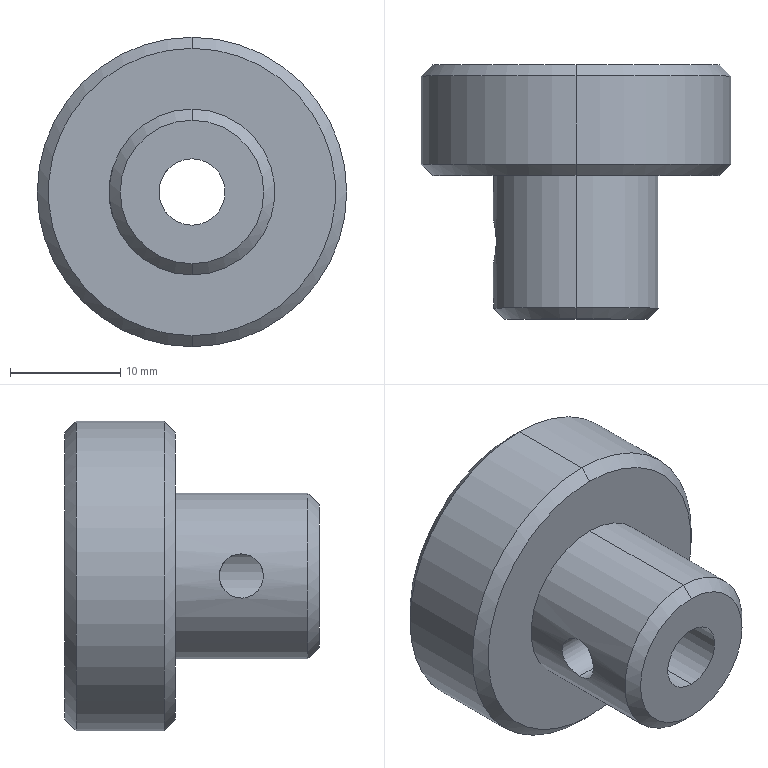Part | SolidWorks | features ICE 2, Chamfer 1, Extrusion 1 | 1 solid | 17 faces | box 28 x 23 x 28 mm | volume 7638 mm3 | cylinder 8 | cone 6 | plane 3 | commonest cylinder face diameters 4 x2 6 x2 15 x2 28 x2
STEP:
#1=CARTESIAN_POINT('',(-7.228,7.04,2.));
#2=VERTEX_POINT('',#1);
#3=CARTESIAN_POINT('',(-7.228,7.04,-2.));
#4=VERTEX_POINT('',#3);
#5=CARTESIAN_POINT('',(-7.228,7.04,2.));
#6=CARTESIAN_POINT('',(-7.228,6.778,2.));
#7=CARTESIAN_POINT('',(-7.244,6.514,1.947));
#8=CARTESIAN_POINT('',(-7.282,6.152,1.797));
#9=CARTESIAN_POINT('',(-7.297,6.035,1.734));
#10=CARTESIAN_POINT('',(-7.33,5.819,1.589));
#11=CARTESIAN_POINT('',(-7.348,5.718,1.507));
#12=CARTESIAN_POINT('',(-7.383,5.534,1.323));
#13=CARTESIAN_POINT('',(-7.401,5.45,1.22));
#14=CARTESIAN_POINT('',(-7.433,5.305,1.005));
#15=CARTESIAN_POINT('',(-7.448,5.244,0.8899));
#16=CARTESIAN_POINT('',(-7.473,5.142,0.6464));
#17=CARTESIAN_POINT('',(-7.483,5.104,0.5208));
#18=CARTESIAN_POINT('',(-7.496,5.053,0.2647));
#19=CARTESIAN_POINT('',(-7.5,5.04,0.1323));
#20=CARTESIAN_POINT('',(-7.5,5.04,-0.1314));
#21=CARTESIAN_POINT('',(-7.497,5.052,-0.2616));
#22=CARTESIAN_POINT('',(-7.483,5.104,-0.5188));
#23=CARTESIAN_POINT('',(-7.473,5.142,-0.6464));
#24=CARTESIAN_POINT('',(-7.436,5.293,-1.008));
#25=CARTESIAN_POINT('',(-7.401,5.441,-1.23));
#26=CARTESIAN_POINT('',(-7.348,5.717,-1.505));
#27=CARTESIAN_POINT('',(-7.33,5.818,-1.589));
#28=CARTESIAN_POINT('',(-7.297,6.036,-1.735));
#29=CARTESIAN_POINT('',(-7.282,6.15,-1.796));
#30=CARTESIAN_POINT('',(-7.256,6.391,-1.896));
#31=CARTESIAN_POINT('',(-7.246,6.519,-1.935));
#32=CARTESIAN_POINT('',(-7.232,6.776,-1.987));
#33=CARTESIAN_POINT('',(-7.228,6.907,-2.));
#34=CARTESIAN_POINT('',(-7.228,7.04,-2.));
#35=B_SPLINE_CURVE_WITH_KNOTS('',3,(#5,#6,#7,#8,#9,#10,#11,#12,#13,#14,#15,#16,#17,#18,#19,#20,#21,#22,#23,#24,#25,#26,#27,#28,#29,#30,#31,#32,#33,#34),.UNSPECIFIED.,.F.,.F.,(4,2,2,2,2,2,2,2,2,2,2,2,2,2,4),(0.006281,0.007066,0.007459,0.007851,0.008244,0.008636,0.009029,0.009421,0.009814,0.01021,0.01099,0.01138,0.01178,0.01217,0.01256),.UNSPECIFIED.);
#36=EDGE_CURVE('',#2,#4,#35,.T.);
#37=ORIENTED_EDGE('',*,*,#36,.F.);
#38=CARTESIAN_POINT('',(-2.236,7.04,2.));
#39=VERTEX_POINT('',#38);
#40=CARTESIAN_POINT('',(-15.,7.04,2.));
#41=DIRECTION('',(1.,0.,0.));
#42=VECTOR('',#41,1000.);
#43=LINE('',#40,#42);
#44=EDGE_CURVE('',#2,#39,#43,.T.);
#45=ORIENTED_EDGE('',*,*,#44,.T.);
#46=CARTESIAN_POINT('',(-2.236,7.04,-2.));
#47=VERTEX_POINT('',#46);
#48=CARTESIAN_POINT('',(-2.236,7.04,2.));
#49=CARTESIAN_POINT('',(-2.236,6.769,2.));
#50=CARTESIAN_POINT('',(-2.289,6.501,1.944));
#51=CARTESIAN_POINT('',(-2.446,6.022,1.741));
#52=CARTESIAN_POINT('',(-2.548,5.81,1.597));
#53=CARTESIAN_POINT('',(-2.692,5.539,1.329));
#54=CARTESIAN_POINT('',(-2.738,5.459,1.231));
#55=CARTESIAN_POINT('',(-2.823,5.315,1.02));
#56=CARTESIAN_POINT('',(-2.863,5.251,0.905));
#57=CARTESIAN_POINT('',(-2.928,5.148,0.6631));
#58=CARTESIAN_POINT('',(-2.955,5.108,0.5369));
#59=CARTESIAN_POINT('',(-2.991,5.054,0.2726));
#60=CARTESIAN_POINT('',(-3.,5.04,0.137));
#61=CARTESIAN_POINT('',(-3.,5.039,-0.1323));
#62=CARTESIAN_POINT('',(-2.991,5.053,-0.2692));
#63=CARTESIAN_POINT('',(-2.955,5.107,-0.5325));
#64=CARTESIAN_POINT('',(-2.929,5.147,-0.6592));
#65=CARTESIAN_POINT('',(-2.864,5.25,-0.9032));
#66=CARTESIAN_POINT('',(-2.825,5.313,-1.017));
#67=CARTESIAN_POINT('',(-2.739,5.457,-1.23));
#68=CARTESIAN_POINT('',(-2.691,5.54,-1.329));
#69=CARTESIAN_POINT('',(-2.596,5.719,-1.507));
#70=CARTESIAN_POINT('',(-2.547,5.816,-1.587));
#71=CARTESIAN_POINT('',(-2.453,6.028,-1.73));
#72=CARTESIAN_POINT('',(-2.407,6.141,-1.792));
#73=CARTESIAN_POINT('',(-2.329,6.379,-1.892));
#74=CARTESIAN_POINT('',(-2.295,6.506,-1.932));
#75=CARTESIAN_POINT('',(-2.249,6.769,-1.986));
#76=CARTESIAN_POINT('',(-2.236,6.903,-2.));
#77=CARTESIAN_POINT('',(-2.236,7.04,-2.));
#78=B_SPLINE_CURVE_WITH_KNOTS('',3,(#48,#49,#50,#51,#52,#53,#54,#55,#56,#57,#58,#59,#60,#61,#62,#63,#64,#65,#66,#67,#68,#69,#70,#71,#72,#73,#74,#75,#76,#77),.UNSPECIFIED.,.F.,.F.,(4,2,2,2,2,2,2,2,2,2,2,2,2,2,4),(0.00646,0.007265,0.00807,0.008472,0.008875,0.009277,0.00968,0.01008,0.01048,0.01089,0.01129,0.01169,0.0121,0.0125,0.0129),.UNSPECIFIED.);
#79=EDGE_CURVE('',#39,#47,#78,.T.);
#80=ORIENTED_EDGE('',*,*,#79,.T.);
#81=CARTESIAN_POINT('',(-15.,7.04,-2.));
#82=DIRECTION('',(1.,0.,0.));
#83=VECTOR('',#82,1000.);
#84=LINE('',#81,#83);
#85=EDGE_CURVE('',#4,#47,#84,.T.);
#86=ORIENTED_EDGE('',*,*,#85,.F.);
#87=EDGE_LOOP('',(#37,#45,#80,#86));
#88=FACE_OUTER_BOUND('',#87,.T.);
#89=CARTESIAN_POINT('',(-15.,7.04,0.));
#90=DIRECTION('',(1.,0.,0.));
#91=DIRECTION('',(0.,0.,-1.));
#92=AXIS2_PLACEMENT_3D('',#89,#90,#91);
#93=CYLINDRICAL_SURFACE('',#92,2.);
#94=ADVANCED_FACE('',(#88),#93,.F.);
#95=CARTESIAN_POINT('',(0.,0.,-6.5));
#96=VERTEX_POINT('',#95);
#97=CARTESIAN_POINT('',(0.,0.,6.5));
#98=VERTEX_POINT('',#97);
#99=CARTESIAN_POINT('',(0.,0.,0.));
#100=DIRECTION('',(0.,-1.,0.));
#101=DIRECTION('',(0.,0.,1.));
#102=AXIS2_PLACEMENT_3D('',#99,#100,#101);
#103=CIRCLE('',#102,6.5);
#104=EDGE_CURVE('',#96,#98,#103,.T.);
#105=ORIENTED_EDGE('',*,*,#104,.F.);
#106=CARTESIAN_POINT('',(0.,1.,-7.5));
#107=VERTEX_POINT('',#106);
#108=CARTESIAN_POINT('',(0.,1.,-7.5));
#109=DIRECTION('',(0.,0.7071,-0.7071));
#110=VECTOR('',#109,1000.);
#111=LINE('',#108,#110);
#112=EDGE_CURVE('',#96,#107,#111,.T.);
#113=ORIENTED_EDGE('',*,*,#112,.T.);
#114=CARTESIAN_POINT('',(0.,1.,7.5));
#115=VERTEX_POINT('',#114);
#116=CARTESIAN_POINT('',(0.,1.,0.));
#117=DIRECTION('',(0.,1.,0.));
#118=DIRECTION('',(0.,0.,1.));
#119=AXIS2_PLACEMENT_3D('',#116,#117,#118);
#120=CIRCLE('',#119,7.5);
#121=EDGE_CURVE('',#115,#107,#120,.T.);
#122=ORIENTED_EDGE('',*,*,#121,.F.);
#123=CARTESIAN_POINT('',(0.,1.,7.5));
#124=DIRECTION('',(0.,0.7071,0.7071));
#125=VECTOR('',#124,1000.);
#126=LINE('',#123,#125);
#127=EDGE_CURVE('',#98,#115,#126,.T.);
#128=ORIENTED_EDGE('',*,*,#127,.F.);
#129=EDGE_LOOP('',(#105,#113,#122,#128));
#130=FACE_OUTER_BOUND('',#129,.T.);
#131=CARTESIAN_POINT('',(0.,1.,0.));
#132=DIRECTION('',(0.,1.,0.));
#133=DIRECTION('',(0.,0.,1.));
#134=AXIS2_PLACEMENT_3D('',#131,#132,#133);
#135=CONICAL_SURFACE('',#134,7.5,0.7854);
#136=ADVANCED_FACE('',(#130),#135,.T.);
#137=CARTESIAN_POINT('',(0.,13.,-13.));
#138=VERTEX_POINT('',#137);
#139=CARTESIAN_POINT('',(0.,13.,13.));
#140=VERTEX_POINT('',#139);
#141=CARTESIAN_POINT('',(0.,13.,0.));
#142=DIRECTION('',(0.,-1.,0.));
#143=DIRECTION('',(0.,0.,1.));
#144=AXIS2_PLACEMENT_3D('',#141,#142,#143);
#145=CIRCLE('',#144,13.);
#146=EDGE_CURVE('',#138,#140,#145,.T.);
#147=ORIENTED_EDGE('',*,*,#146,.F.);
#148=CARTESIAN_POINT('',(0.,14.,-14.));
#149=VERTEX_POINT('',#148);
#150=CARTESIAN_POINT('',(0.,14.,-14.));
#151=DIRECTION('',(0.,0.7071,-0.7071));
#152=VECTOR('',#151,1000.);
#153=LINE('',#150,#152);
#154=EDGE_CURVE('',#138,#149,#153,.T.);
#155=ORIENTED_EDGE('',*,*,#154,.T.);
#156=CARTESIAN_POINT('',(0.,14.,14.));
#157=VERTEX_POINT('',#156);
#158=CARTESIAN_POINT('',(0.,14.,0.));
#159=DIRECTION('',(0.,1.,0.));
#160=DIRECTION('',(0.,0.,1.));
#161=AXIS2_PLACEMENT_3D('',#158,#159,#160);
#162=CIRCLE('',#161,14.);
#163=EDGE_CURVE('',#157,#149,#162,.T.);
#164=ORIENTED_EDGE('',*,*,#163,.F.);
#165=CARTESIAN_POINT('',(0.,14.,14.));
#166=DIRECTION('',(0.,0.7071,0.7071));
#167=VECTOR('',#166,1000.);
#168=LINE('',#165,#167);
#169=EDGE_CURVE('',#140,#157,#168,.T.);
#170=ORIENTED_EDGE('',*,*,#169,.F.);
#171=EDGE_LOOP('',(#147,#155,#164,#170));
#172=FACE_OUTER_BOUND('',#171,.T.);
#173=CARTESIAN_POINT('',(0.,14.,0.));
#174=DIRECTION('',(0.,1.,0.));
#175=DIRECTION('',(0.,0.,1.));
#176=AXIS2_PLACEMENT_3D('',#173,#174,#175);
#177=CONICAL_SURFACE('',#176,14.,0.7854);
#178=ADVANCED_FACE('',(#172),#177,.T.);
#179=CARTESIAN_POINT('',(0.,23.,13.));
#180=VERTEX_POINT('',#179);
#181=CARTESIAN_POINT('',(0.,23.,-13.));
#182=VERTEX_POINT('',#181);
#183=CARTESIAN_POINT('',(0.,23.,0.));
#184=DIRECTION('',(0.,1.,0.));
#185=DIRECTION('',(0.,0.,1.));
#186=AXIS2_PLACEMENT_3D('',#183,#184,#185);
#187=CIRCLE('',#186,13.);
#188=EDGE_CURVE('',#180,#182,#187,.T.);
#189=ORIENTED_EDGE('',*,*,#188,.F.);
#190=CARTESIAN_POINT('',(0.,22.,14.));
#191=VERTEX_POINT('',#190);
#192=CARTESIAN_POINT('',(0.,23.,13.));
#193=DIRECTION('',(0.,-0.7071,0.7071));
#194=VECTOR('',#193,1000.);
#195=LINE('',#192,#194);
#196=EDGE_CURVE('',#180,#191,#195,.T.);
#197=ORIENTED_EDGE('',*,*,#196,.T.);
#198=CARTESIAN_POINT('',(0.,22.,-14.));
#199=VERTEX_POINT('',#198);
#200=CARTESIAN_POINT('',(0.,22.,0.));
#201=DIRECTION('',(0.,-1.,0.));
#202=DIRECTION('',(0.,0.,1.));
#203=AXIS2_PLACEMENT_3D('',#200,#201,#202);
#204=CIRCLE('',#203,14.);
#205=EDGE_CURVE('',#199,#191,#204,.T.);
#206=ORIENTED_EDGE('',*,*,#205,.F.);
#207=CARTESIAN_POINT('',(0.,23.,-13.));
#208=DIRECTION('',(0.,-0.7071,-0.7071));
#209=VECTOR('',#208,1000.);
#210=LINE('',#207,#209);
#211=EDGE_CURVE('',#182,#199,#210,.T.);
#212=ORIENTED_EDGE('',*,*,#211,.F.);
#213=EDGE_LOOP('',(#189,#197,#206,#212));
#214=FACE_OUTER_BOUND('',#213,.T.);
#215=CARTESIAN_POINT('',(0.,23.,0.));
#216=DIRECTION('',(0.,-1.,0.));
#217=DIRECTION('',(0.,0.,-1.));
#218=AXIS2_PLACEMENT_3D('',#215,#216,#217);
#219=CONICAL_SURFACE('',#218,13.,0.7854);
#220=ADVANCED_FACE('',(#214),#219,.T.);
#221=ORIENTED_EDGE('',*,*,#163,.T.);
#222=CARTESIAN_POINT('',(0.,13.,-14.));
#223=DIRECTION('',(0.,1.,0.));
#224=VECTOR('',#223,1000.);
#225=LINE('',#222,#224);
#226=EDGE_CURVE('',#149,#199,#225,.T.);
#227=ORIENTED_EDGE('',*,*,#226,.T.);
#228=ORIENTED_EDGE('',*,*,#205,.T.);
#229=CARTESIAN_POINT('',(0.,13.,14.));
#230=DIRECTION('',(0.,1.,0.));
#231=VECTOR('',#230,1000.);
#232=LINE('',#229,#231);
#233=EDGE_CURVE('',#157,#191,#232,.T.);
#234=ORIENTED_EDGE('',*,*,#233,.F.);
#235=EDGE_LOOP('',(#221,#227,#228,#234));
#236=FACE_OUTER_BOUND('',#235,.T.);
#237=CARTESIAN_POINT('',(0.,13.,0.));
#238=DIRECTION('',(0.,1.,0.));
#239=DIRECTION('',(0.,0.,1.));
#240=AXIS2_PLACEMENT_3D('',#237,#238,#239);
#241=CYLINDRICAL_SURFACE('',#240,14.);
#242=ADVANCED_FACE('',(#236),#241,.T.);
#243=CARTESIAN_POINT('',(-2.236,7.04,-2.));
#244=CARTESIAN_POINT('',(-2.236,7.177,-2.));
#245=CARTESIAN_POINT('',(-2.249,7.31,-1.986));
#246=CARTESIAN_POINT('',(-2.295,7.571,-1.933));
#247=CARTESIAN_POINT('',(-2.328,7.698,-1.893));
#248=CARTESIAN_POINT('',(-2.446,8.056,-1.742));
#249=CARTESIAN_POINT('',(-2.547,8.269,-1.597));
#250=CARTESIAN_POINT('',(-2.691,8.539,-1.33));
#251=CARTESIAN_POINT('',(-2.738,8.621,-1.231));
#252=CARTESIAN_POINT('',(-2.824,8.765,-1.019));
#253=CARTESIAN_POINT('',(-2.863,8.827,-0.9064));
#254=CARTESIAN_POINT('',(-2.928,8.93,-0.6656));
#255=CARTESIAN_POINT('',(-2.955,8.971,-0.5362));
#256=CARTESIAN_POINT('',(-2.99,9.025,-0.275));
#257=CARTESIAN_POINT('',(-3.,9.039,-0.1417));
#258=CARTESIAN_POINT('',(-3.,9.04,0.1311));
#259=CARTESIAN_POINT('',(-2.991,9.026,0.2667));
#260=CARTESIAN_POINT('',(-2.956,8.973,0.5294));
#261=CARTESIAN_POINT('',(-2.929,8.933,0.6589));
#262=CARTESIAN_POINT('',(-2.832,8.779,1.022));
#263=CARTESIAN_POINT('',(-2.74,8.63,1.238));
#264=CARTESIAN_POINT('',(-2.596,8.361,1.507));
#265=CARTESIAN_POINT('',(-2.547,8.262,1.588));
#266=CARTESIAN_POINT('',(-2.453,8.052,1.73));
#267=CARTESIAN_POINT('',(-2.408,7.94,1.791));
#268=CARTESIAN_POINT('',(-2.329,7.701,1.892));
#269=CARTESIAN_POINT('',(-2.295,7.574,1.932));
#270=CARTESIAN_POINT('',(-2.249,7.312,1.986));
#271=CARTESIAN_POINT('',(-2.236,7.175,2.));
#272=CARTESIAN_POINT('',(-2.236,7.04,2.));
#273=B_SPLINE_CURVE_WITH_KNOTS('',3,(#243,#244,#245,#246,#247,#248,#249,#250,#251,#252,#253,#254,#255,#256,#257,#258,#259,#260,#261,#262,#263,#264,#265,#266,#267,#268,#269,#270,#271,#272),.UNSPECIFIED.,.F.,.F.,(4,2,2,2,2,2,2,2,2,2,2,2,2,2,4),(0.,0.0004037,0.0008075,0.001615,0.002019,0.002422,0.002826,0.00323,0.003634,0.004037,0.004845,0.005248,0.005652,0.006056,0.00646),.UNSPECIFIED.);
#274=EDGE_CURVE('',#47,#39,#273,.T.);
#275=ORIENTED_EDGE('',*,*,#274,.F.);
#276=ORIENTED_EDGE('',*,*,#79,.F.);
#277=EDGE_LOOP('',(#275,#276));
#278=FACE_BOUND('',#277,.T.);
#279=CARTESIAN_POINT('',(0.,23.,-3.));
#280=VERTEX_POINT('',#279);
#281=CARTESIAN_POINT('',(0.,23.,3.));
#282=VERTEX_POINT('',#281);
#283=CARTESIAN_POINT('',(0.,23.,0.));
#284=DIRECTION('',(0.,1.,0.));
#285=DIRECTION('',(0.,0.,1.));
#286=AXIS2_PLACEMENT_3D('',#283,#284,#285);
#287=CIRCLE('',#286,3.);
#288=EDGE_CURVE('',#280,#282,#287,.T.);
#289=ORIENTED_EDGE('',*,*,#288,.T.);
#290=CARTESIAN_POINT('',(0.,0.,3.));
#291=VERTEX_POINT('',#290);
#292=CARTESIAN_POINT('',(0.,23.,3.));
#293=DIRECTION('',(0.,-1.,0.));
#294=VECTOR('',#293,1000.);
#295=LINE('',#292,#294);
#296=EDGE_CURVE('',#282,#291,#295,.T.);
#297=ORIENTED_EDGE('',*,*,#296,.T.);
#298=CARTESIAN_POINT('',(0.,0.,-3.));
#299=VERTEX_POINT('',#298);
#300=CARTESIAN_POINT('',(0.,0.,0.));
#301=DIRECTION('',(0.,1.,0.));
#302=DIRECTION('',(0.,0.,1.));
#303=AXIS2_PLACEMENT_3D('',#300,#301,#302);
#304=CIRCLE('',#303,3.);
#305=EDGE_CURVE('',#299,#291,#304,.T.);
#306=ORIENTED_EDGE('',*,*,#305,.F.);
#307=CARTESIAN_POINT('',(0.,23.,-3.));
#308=DIRECTION('',(0.,-1.,0.));
#309=VECTOR('',#308,1000.);
#310=LINE('',#307,#309);
#311=EDGE_CURVE('',#280,#299,#310,.T.);
#312=ORIENTED_EDGE('',*,*,#311,.F.);
#313=EDGE_LOOP('',(#289,#297,#306,#312));
#314=FACE_OUTER_BOUND('',#313,.T.);
#315=CARTESIAN_POINT('',(0.,23.,0.));
#316=DIRECTION('',(0.,-1.,0.));
#317=DIRECTION('',(0.,0.,-1.));
#318=AXIS2_PLACEMENT_3D('',#315,#316,#317);
#319=CYLINDRICAL_SURFACE('',#318,3.);
#320=ADVANCED_FACE('',(#278,#314),#319,.F.);
#321=CARTESIAN_POINT('',(0.,13.,7.5));
#322=VERTEX_POINT('',#321);
#323=CARTESIAN_POINT('',(0.,13.,-7.5));
#324=VERTEX_POINT('',#323);
#325=CARTESIAN_POINT('',(0.,13.,0.));
#326=DIRECTION('',(0.,1.,0.));
#327=DIRECTION('',(0.,0.,1.));
#328=AXIS2_PLACEMENT_3D('',#325,#326,#327);
#329=CIRCLE('',#328,7.5);
#330=EDGE_CURVE('',#322,#324,#329,.T.);
#331=ORIENTED_EDGE('',*,*,#330,.F.);
#332=CARTESIAN_POINT('',(0.,23.,7.5));
#333=DIRECTION('',(0.,-1.,0.));
#334=VECTOR('',#333,1000.);
#335=LINE('',#332,#334);
#336=EDGE_CURVE('',#322,#115,#335,.T.);
#337=ORIENTED_EDGE('',*,*,#336,.T.);
#338=ORIENTED_EDGE('',*,*,#121,.T.);
#339=CARTESIAN_POINT('',(0.,23.,-7.5));
#340=DIRECTION('',(0.,-1.,0.));
#341=VECTOR('',#340,1000.);
#342=LINE('',#339,#341);
#343=EDGE_CURVE('',#324,#107,#342,.T.);
#344=ORIENTED_EDGE('',*,*,#343,.F.);
#345=EDGE_LOOP('',(#331,#337,#338,#344));
#346=FACE_OUTER_BOUND('',#345,.T.);
#347=CARTESIAN_POINT('',(0.,23.,0.));
#348=DIRECTION('',(0.,-1.,0.));
#349=DIRECTION('',(0.,0.,-1.));
#350=AXIS2_PLACEMENT_3D('',#347,#348,#349);
#351=CYLINDRICAL_SURFACE('',#350,7.5);
#352=ADVANCED_FACE('',(#346),#351,.T.);
#353=ORIENTED_EDGE('',*,*,#336,.F.);
#354=CARTESIAN_POINT('',(0.,13.,0.));
#355=DIRECTION('',(0.,1.,0.));
#356=DIRECTION('',(0.,0.,1.));
#357=AXIS2_PLACEMENT_3D('',#354,#355,#356);
#358=CIRCLE('',#357,7.5);
#359=EDGE_CURVE('',#324,#322,#358,.T.);
#360=ORIENTED_EDGE('',*,*,#359,.F.);
#361=ORIENTED_EDGE('',*,*,#343,.T.);
#362=CARTESIAN_POINT('',(0.,1.,0.));
#363=DIRECTION('',(0.,1.,0.));
#364=DIRECTION('',(0.,0.,1.));
#365=AXIS2_PLACEMENT_3D('',#362,#363,#364);
#366=CIRCLE('',#365,7.5);
#367=EDGE_CURVE('',#107,#115,#366,.T.);
#368=ORIENTED_EDGE('',*,*,#367,.T.);
#369=EDGE_LOOP('',(#353,#360,#361,#368));
#370=FACE_OUTER_BOUND('',#369,.T.);
#371=CARTESIAN_POINT('',(-7.228,7.04,-2.));
#372=CARTESIAN_POINT('',(-7.228,7.172,-2.));
#373=CARTESIAN_POINT('',(-7.232,7.303,-1.987));
#374=CARTESIAN_POINT('',(-7.246,7.559,-1.936));
#375=CARTESIAN_POINT('',(-7.256,7.687,-1.897));
#376=CARTESIAN_POINT('',(-7.282,7.929,-1.796));
#377=CARTESIAN_POINT('',(-7.297,8.043,-1.735));
#378=CARTESIAN_POINT('',(-7.33,8.26,-1.59));
#379=CARTESIAN_POINT('',(-7.348,8.362,-1.506));
#380=CARTESIAN_POINT('',(-7.401,8.638,-1.23));
#381=CARTESIAN_POINT('',(-7.436,8.787,-1.008));
#382=CARTESIAN_POINT('',(-7.473,8.936,-0.6474));
#383=CARTESIAN_POINT('',(-7.483,8.975,-0.5206));
#384=CARTESIAN_POINT('',(-7.497,9.027,-0.2622));
#385=CARTESIAN_POINT('',(-7.5,9.04,-0.132));
#386=CARTESIAN_POINT('',(-7.5,9.04,0.1303));
#387=CARTESIAN_POINT('',(-7.496,9.027,0.2635));
#388=CARTESIAN_POINT('',(-7.483,8.975,0.5205));
#389=CARTESIAN_POINT('',(-7.473,8.937,0.6455));
#390=CARTESIAN_POINT('',(-7.436,8.786,1.01));
#391=CARTESIAN_POINT('',(-7.401,8.638,1.23));
#392=CARTESIAN_POINT('',(-7.348,8.361,1.507));
#393=CARTESIAN_POINT('',(-7.33,8.26,1.59));
#394=CARTESIAN_POINT('',(-7.297,8.044,1.734));
#395=CARTESIAN_POINT('',(-7.282,7.927,1.797));
#396=CARTESIAN_POINT('',(-7.256,7.686,1.897));
#397=CARTESIAN_POINT('',(-7.246,7.561,1.935));
#398=CARTESIAN_POINT('',(-7.232,7.303,1.987));
#399=CARTESIAN_POINT('',(-7.228,7.171,2.));
#400=CARTESIAN_POINT('',(-7.228,7.04,2.));
#401=B_SPLINE_CURVE_WITH_KNOTS('',3,(#371,#372,#373,#374,#375,#376,#377,#378,#379,#380,#381,#382,#383,#384,#385,#386,#387,#388,#389,#390,#391,#392,#393,#394,#395,#396,#397,#398,#399,#400),.UNSPECIFIED.,.F.,.F.,(4,2,2,2,2,2,2,2,2,2,2,2,2,2,4),(0.,0.0003926,0.0007852,0.001178,0.00157,0.002356,0.002748,0.003141,0.003533,0.003926,0.004711,0.005104,0.005496,0.005889,0.006281),.UNSPECIFIED.);
#402=EDGE_CURVE('',#4,#2,#401,.T.);
#403=ORIENTED_EDGE('',*,*,#402,.T.);
#404=ORIENTED_EDGE('',*,*,#36,.T.);
#405=EDGE_LOOP('',(#403,#404));
#406=FACE_BOUND('',#405,.T.);
#407=CARTESIAN_POINT('',(0.,23.,0.));
#408=DIRECTION('',(0.,-1.,0.));
#409=DIRECTION('',(0.,0.,-1.));
#410=AXIS2_PLACEMENT_3D('',#407,#408,#409);
#411=CYLINDRICAL_SURFACE('',#410,7.5);
#412=ADVANCED_FACE('',(#370,#406),#411,.T.);
#413=CARTESIAN_POINT('',(0.,23.,0.));
#414=DIRECTION('',(0.,1.,0.));
#415=DIRECTION('',(0.,0.,1.));
#416=AXIS2_PLACEMENT_3D('',#413,#414,#415);
#417=CIRCLE('',#416,13.);
#418=EDGE_CURVE('',#182,#180,#417,.T.);
#419=ORIENTED_EDGE('',*,*,#418,.T.);
#420=ORIENTED_EDGE('',*,*,#188,.T.);
#421=EDGE_LOOP('',(#419,#420));
#422=FACE_OUTER_BOUND('',#421,.T.);
#423=ORIENTED_EDGE('',*,*,#288,.F.);
#424=CARTESIAN_POINT('',(0.,23.,0.));
#425=DIRECTION('',(0.,1.,0.));
#426=DIRECTION('',(0.,0.,1.));
#427=AXIS2_PLACEMENT_3D('',#424,#425,#426);
#428=CIRCLE('',#427,3.);
#429=EDGE_CURVE('',#282,#280,#428,.T.);
#430=ORIENTED_EDGE('',*,*,#429,.F.);
#431=EDGE_LOOP('',(#423,#430));
#432=FACE_BOUND('',#431,.T.);
#433=CARTESIAN_POINT('',(0.,23.,0.));
#434=DIRECTION('',(0.,1.,0.));
#435=DIRECTION('',(0.,0.,1.));
#436=AXIS2_PLACEMENT_3D('',#433,#434,#435);
#437=PLANE('',#436);
#438=ADVANCED_FACE('',(#422,#432),#437,.T.);
#439=CARTESIAN_POINT('',(0.,0.,0.));
#440=DIRECTION('',(0.,-1.,0.));
#441=DIRECTION('',(0.,0.,1.));
#442=AXIS2_PLACEMENT_3D('',#439,#440,#441);
#443=CIRCLE('',#442,6.5);
#444=EDGE_CURVE('',#98,#96,#443,.T.);
#445=ORIENTED_EDGE('',*,*,#444,.T.);
#446=ORIENTED_EDGE('',*,*,#104,.T.);
#447=EDGE_LOOP('',(#445,#446));
#448=FACE_OUTER_BOUND('',#447,.T.);
#449=ORIENTED_EDGE('',*,*,#305,.T.);
#450=CARTESIAN_POINT('',(0.,0.,0.));
#451=DIRECTION('',(0.,1.,0.));
#452=DIRECTION('',(0.,0.,1.));
#453=AXIS2_PLACEMENT_3D('',#450,#451,#452);
#454=CIRCLE('',#453,3.);
#455=EDGE_CURVE('',#291,#299,#454,.T.);
#456=ORIENTED_EDGE('',*,*,#455,.T.);
#457=EDGE_LOOP('',(#449,#456));
#458=FACE_BOUND('',#457,.T.);
#459=CARTESIAN_POINT('',(0.,0.,0.));
#460=DIRECTION('',(0.,1.,0.));
#461=DIRECTION('',(0.,0.,1.));
#462=AXIS2_PLACEMENT_3D('',#459,#460,#461);
#463=PLANE('',#462);
#464=ADVANCED_FACE('',(#448,#458),#463,.F.);
#465=ORIENTED_EDGE('',*,*,#296,.F.);
#466=ORIENTED_EDGE('',*,*,#429,.T.);
#467=ORIENTED_EDGE('',*,*,#311,.T.);
#468=ORIENTED_EDGE('',*,*,#455,.F.);
#469=EDGE_LOOP('',(#465,#466,#467,#468));
#470=FACE_OUTER_BOUND('',#469,.T.);
#471=CARTESIAN_POINT('',(0.,23.,0.));
#472=DIRECTION('',(0.,-1.,0.));
#473=DIRECTION('',(0.,0.,-1.));
#474=AXIS2_PLACEMENT_3D('',#471,#472,#473);
#475=CYLINDRICAL_SURFACE('',#474,3.);
#476=ADVANCED_FACE('',(#470),#475,.F.);
#477=CARTESIAN_POINT('',(0.,13.,0.));
#478=DIRECTION('',(0.,-1.,0.));
#479=DIRECTION('',(0.,0.,1.));
#480=AXIS2_PLACEMENT_3D('',#477,#478,#479);
#481=CIRCLE('',#480,13.);
#482=EDGE_CURVE('',#140,#138,#481,.T.);
#483=ORIENTED_EDGE('',*,*,#482,.T.);
#484=ORIENTED_EDGE('',*,*,#146,.T.);
#485=EDGE_LOOP('',(#483,#484));
#486=FACE_OUTER_BOUND('',#485,.T.);
#487=ORIENTED_EDGE('',*,*,#359,.T.);
#488=ORIENTED_EDGE('',*,*,#330,.T.);
#489=EDGE_LOOP('',(#487,#488));
#490=FACE_BOUND('',#489,.T.);
#491=CARTESIAN_POINT('',(0.,13.,0.));
#492=DIRECTION('',(0.,1.,0.));
#493=DIRECTION('',(0.,0.,1.));
#494=AXIS2_PLACEMENT_3D('',#491,#492,#493);
#495=PLANE('',#494);
#496=ADVANCED_FACE('',(#486,#490),#495,.F.);
#497=ORIENTED_EDGE('',*,*,#226,.F.);
#498=CARTESIAN_POINT('',(0.,14.,0.));
#499=DIRECTION('',(0.,1.,0.));
#500=DIRECTION('',(0.,0.,1.));
#501=AXIS2_PLACEMENT_3D('',#498,#499,#500);
#502=CIRCLE('',#501,14.);
#503=EDGE_CURVE('',#149,#157,#502,.T.);
#504=ORIENTED_EDGE('',*,*,#503,.T.);
#505=ORIENTED_EDGE('',*,*,#233,.T.);
#506=CARTESIAN_POINT('',(0.,22.,0.));
#507=DIRECTION('',(0.,-1.,0.));
#508=DIRECTION('',(0.,0.,1.));
#509=AXIS2_PLACEMENT_3D('',#506,#507,#508);
#510=CIRCLE('',#509,14.);
#511=EDGE_CURVE('',#191,#199,#510,.T.);
#512=ORIENTED_EDGE('',*,*,#511,.T.);
#513=EDGE_LOOP('',(#497,#504,#505,#512));
#514=FACE_OUTER_BOUND('',#513,.T.);
#515=CARTESIAN_POINT('',(0.,13.,0.));
#516=DIRECTION('',(0.,1.,0.));
#517=DIRECTION('',(0.,0.,1.));
#518=AXIS2_PLACEMENT_3D('',#515,#516,#517);
#519=CYLINDRICAL_SURFACE('',#518,14.);
#520=ADVANCED_FACE('',(#514),#519,.T.);
#521=ORIENTED_EDGE('',*,*,#196,.F.);
#522=ORIENTED_EDGE('',*,*,#418,.F.);
#523=ORIENTED_EDGE('',*,*,#211,.T.);
#524=ORIENTED_EDGE('',*,*,#511,.F.);
#525=EDGE_LOOP('',(#521,#522,#523,#524));
#526=FACE_OUTER_BOUND('',#525,.T.);
#527=CARTESIAN_POINT('',(0.,23.,0.));
#528=DIRECTION('',(0.,-1.,0.));
#529=DIRECTION('',(0.,0.,-1.));
#530=AXIS2_PLACEMENT_3D('',#527,#528,#529);
#531=CONICAL_SURFACE('',#530,13.,0.7854);
#532=ADVANCED_FACE('',(#526),#531,.T.);
#533=ORIENTED_EDGE('',*,*,#154,.F.);
#534=ORIENTED_EDGE('',*,*,#482,.F.);
#535=ORIENTED_EDGE('',*,*,#169,.T.);
#536=ORIENTED_EDGE('',*,*,#503,.F.);
#537=EDGE_LOOP('',(#533,#534,#535,#536));
#538=FACE_OUTER_BOUND('',#537,.T.);
#539=CARTESIAN_POINT('',(0.,14.,0.));
#540=DIRECTION('',(0.,1.,0.));
#541=DIRECTION('',(0.,0.,1.));
#542=AXIS2_PLACEMENT_3D('',#539,#540,#541);
#543=CONICAL_SURFACE('',#542,14.,0.7854);
#544=ADVANCED_FACE('',(#538),#543,.T.);
#545=ORIENTED_EDGE('',*,*,#112,.F.);
#546=ORIENTED_EDGE('',*,*,#444,.F.);
#547=ORIENTED_EDGE('',*,*,#127,.T.);
#548=ORIENTED_EDGE('',*,*,#367,.F.);
#549=EDGE_LOOP('',(#545,#546,#547,#548));
#550=FACE_OUTER_BOUND('',#549,.T.);
#551=CARTESIAN_POINT('',(0.,1.,0.));
#552=DIRECTION('',(0.,1.,0.));
#553=DIRECTION('',(0.,0.,1.));
#554=AXIS2_PLACEMENT_3D('',#551,#552,#553);
#555=CONICAL_SURFACE('',#554,7.5,0.7854);
#556=ADVANCED_FACE('',(#550),#555,.T.);
#557=ORIENTED_EDGE('',*,*,#44,.F.);
#558=ORIENTED_EDGE('',*,*,#402,.F.);
#559=ORIENTED_EDGE('',*,*,#85,.T.);
#560=ORIENTED_EDGE('',*,*,#274,.T.);
#561=EDGE_LOOP('',(#557,#558,#559,#560));
#562=FACE_OUTER_BOUND('',#561,.T.);
#563=CARTESIAN_POINT('',(-15.,7.04,0.));
#564=DIRECTION('',(1.,0.,0.));
#565=DIRECTION('',(0.,0.,-1.));
#566=AXIS2_PLACEMENT_3D('',#563,#564,#565);
#567=CYLINDRICAL_SURFACE('',#566,2.);
#568=ADVANCED_FACE('',(#562),#567,.F.);
#569=CLOSED_SHELL('',(#94,#136,#178,#220,#242,#320,#352,#412,#438,#464,#476,#496,#520,#532,#544,#556,#568));
#570=MANIFOLD_SOLID_BREP('',#569);
#571=CARTESIAN_POINT('',(0.,0.,0.));
#572=DIRECTION('',(0.,0.,1.));
#573=DIRECTION('',(1.,0.,0.));
#574=AXIS2_PLACEMENT_3D('',#571,#572,#573);
#575=(LENGTH_UNIT()NAMED_UNIT(*)SI_UNIT(.MILLI.,.METRE.));
#576=UNCERTAINTY_MEASURE_WITH_UNIT(LENGTH_MEASURE(0.00001),#575,'','');
#577=(NAMED_UNIT(*)PLANE_ANGLE_UNIT()SI_UNIT($,.RADIAN.));
#578=(NAMED_UNIT(*)SI_UNIT($,.STERADIAN.)SOLID_ANGLE_UNIT());
#579=(GEOMETRIC_REPRESENTATION_CONTEXT(3)GLOBAL_UNCERTAINTY_ASSIGNED_CONTEXT((#576))GLOBAL_UNIT_ASSIGNED_CONTEXT((#575,#577,#578))REPRESENTATION_CONTEXT('',''));
#580=ADVANCED_BREP_SHAPE_REPRESENTATION('',(#570,#574),#579);